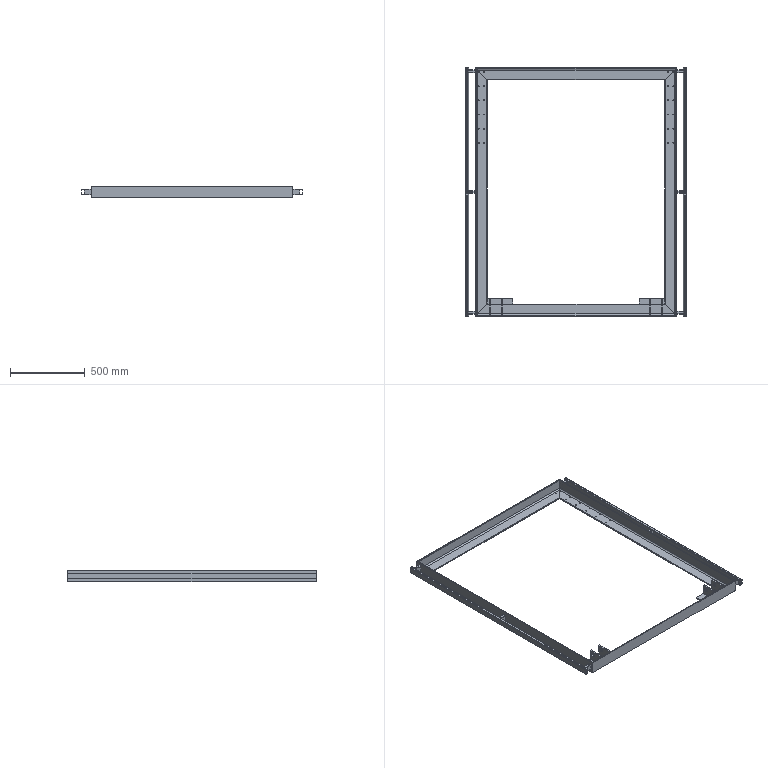Part | STEP file | PN_0001-01-02 Lifting platform base_Default<Machined> | 18 solids | 284 faces | box 1480 x 1665 x 80 mm | volume 7503788 mm3 | plane 148 | cylinder 136 | commonest cylinder face diameters 5 x48 4 x32 8 x32 4.667 x8 18 x8 25 x8